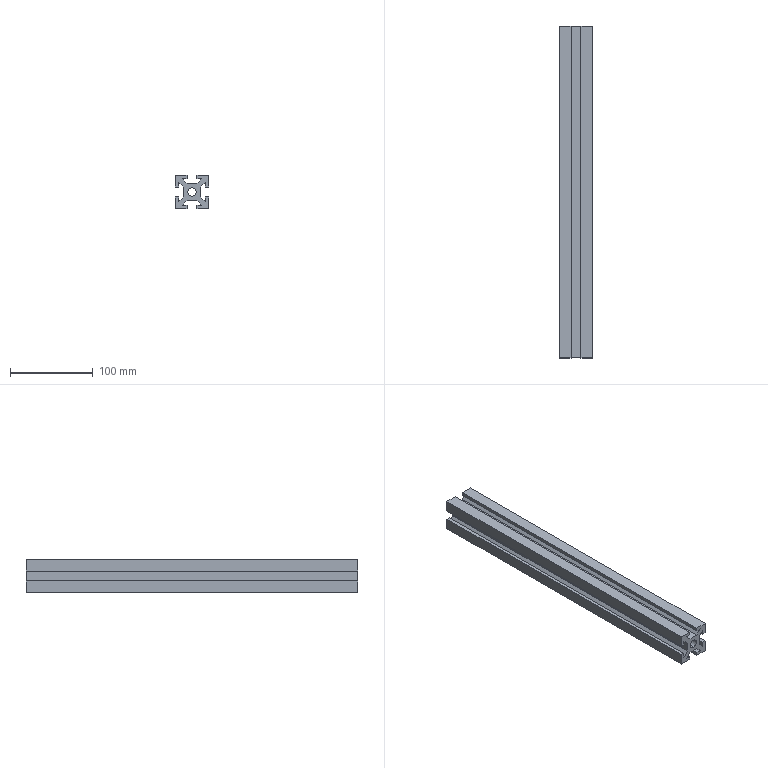Part | SolidWorks | features Extrusion 1 | 1 solid | 40 faces | box 40 x 400 x 40 mm | volume 363643 mm3 | plane 38 | cylinder 2 | commonest cylinder face diameters 10 x2
STEP:
#1=CARTESIAN_POINT('',(0.,400.,-5.));
#2=VERTEX_POINT('',#1);
#3=CARTESIAN_POINT('',(0.,400.,5.));
#4=VERTEX_POINT('',#3);
#5=CARTESIAN_POINT('',(0.,400.,0.));
#6=DIRECTION('',(0.,1.,0.));
#7=DIRECTION('',(0.,0.,1.));
#8=AXIS2_PLACEMENT_3D('',#5,#6,#7);
#9=CIRCLE('',#8,5.);
#10=EDGE_CURVE('',#2,#4,#9,.T.);
#11=ORIENTED_EDGE('',*,*,#10,.T.);
#12=CARTESIAN_POINT('',(0.,0.,5.));
#13=VERTEX_POINT('',#12);
#14=CARTESIAN_POINT('',(0.,400.,5.));
#15=DIRECTION('',(0.,-1.,0.));
#16=VECTOR('',#15,1000.);
#17=LINE('',#14,#16);
#18=EDGE_CURVE('',#4,#13,#17,.T.);
#19=ORIENTED_EDGE('',*,*,#18,.T.);
#20=CARTESIAN_POINT('',(0.,0.,-5.));
#21=VERTEX_POINT('',#20);
#22=CARTESIAN_POINT('',(0.,0.,0.));
#23=DIRECTION('',(0.,1.,0.));
#24=DIRECTION('',(0.,0.,1.));
#25=AXIS2_PLACEMENT_3D('',#22,#23,#24);
#26=CIRCLE('',#25,5.);
#27=EDGE_CURVE('',#21,#13,#26,.T.);
#28=ORIENTED_EDGE('',*,*,#27,.F.);
#29=CARTESIAN_POINT('',(0.,400.,-5.));
#30=DIRECTION('',(0.,-1.,0.));
#31=VECTOR('',#30,1000.);
#32=LINE('',#29,#31);
#33=EDGE_CURVE('',#2,#21,#32,.T.);
#34=ORIENTED_EDGE('',*,*,#33,.F.);
#35=EDGE_LOOP('',(#11,#19,#28,#34));
#36=FACE_OUTER_BOUND('',#35,.T.);
#37=CARTESIAN_POINT('',(0.,400.,0.));
#38=DIRECTION('',(0.,-1.,0.));
#39=DIRECTION('',(0.,0.,-1.));
#40=AXIS2_PLACEMENT_3D('',#37,#38,#39);
#41=CYLINDRICAL_SURFACE('',#40,5.);
#42=ADVANCED_FACE('',(#36),#41,.F.);
#43=CARTESIAN_POINT('',(6.,400.,20.));
#44=VERTEX_POINT('',#43);
#45=CARTESIAN_POINT('',(20.,400.,20.));
#46=VERTEX_POINT('',#45);
#47=CARTESIAN_POINT('',(6.,400.,20.));
#48=DIRECTION('',(1.,0.,0.));
#49=VECTOR('',#48,1000.);
#50=LINE('',#47,#49);
#51=EDGE_CURVE('',#44,#46,#50,.T.);
#52=ORIENTED_EDGE('',*,*,#51,.T.);
#53=CARTESIAN_POINT('',(20.,400.,6.));
#54=VERTEX_POINT('',#53);
#55=CARTESIAN_POINT('',(20.,400.,6.));
#56=DIRECTION('',(0.,0.,-1.));
#57=VECTOR('',#56,1000.);
#58=LINE('',#55,#57);
#59=EDGE_CURVE('',#46,#54,#58,.T.);
#60=ORIENTED_EDGE('',*,*,#59,.T.);
#61=CARTESIAN_POINT('',(16.,400.,6.));
#62=VERTEX_POINT('',#61);
#63=CARTESIAN_POINT('',(16.,400.,6.));
#64=DIRECTION('',(-1.,0.,0.));
#65=VECTOR('',#64,1000.);
#66=LINE('',#63,#65);
#67=EDGE_CURVE('',#54,#62,#66,.T.);
#68=ORIENTED_EDGE('',*,*,#67,.T.);
#69=CARTESIAN_POINT('',(16.,400.,11.757));
#70=VERTEX_POINT('',#69);
#71=CARTESIAN_POINT('',(16.,400.,11.757));
#72=DIRECTION('',(0.,0.,1.));
#73=VECTOR('',#72,1000.);
#74=LINE('',#71,#73);
#75=EDGE_CURVE('',#62,#70,#74,.T.);
#76=ORIENTED_EDGE('',*,*,#75,.T.);
#77=CARTESIAN_POINT('',(10.,400.,5.757));
#78=VERTEX_POINT('',#77);
#79=CARTESIAN_POINT('',(10.,400.,5.757));
#80=DIRECTION('',(-0.7071,0.,-0.7071));
#81=VECTOR('',#80,1000.);
#82=LINE('',#79,#81);
#83=EDGE_CURVE('',#70,#78,#82,.T.);
#84=ORIENTED_EDGE('',*,*,#83,.T.);
#85=CARTESIAN_POINT('',(10.,400.,-5.757));
#86=VERTEX_POINT('',#85);
#87=CARTESIAN_POINT('',(10.,400.,5.757));
#88=DIRECTION('',(0.,0.,-1.));
#89=VECTOR('',#88,1000.);
#90=LINE('',#87,#89);
#91=EDGE_CURVE('',#78,#86,#90,.T.);
#92=ORIENTED_EDGE('',*,*,#91,.T.);
#93=CARTESIAN_POINT('',(16.,400.,-11.757));
#94=VERTEX_POINT('',#93);
#95=CARTESIAN_POINT('',(16.,400.,-11.757));
#96=DIRECTION('',(0.7071,0.,-0.7071));
#97=VECTOR('',#96,1000.);
#98=LINE('',#95,#97);
#99=EDGE_CURVE('',#86,#94,#98,.T.);
#100=ORIENTED_EDGE('',*,*,#99,.T.);
#101=CARTESIAN_POINT('',(16.,400.,-6.));
#102=VERTEX_POINT('',#101);
#103=CARTESIAN_POINT('',(16.,400.,-6.));
#104=DIRECTION('',(0.,0.,1.));
#105=VECTOR('',#104,1000.);
#106=LINE('',#103,#105);
#107=EDGE_CURVE('',#94,#102,#106,.T.);
#108=ORIENTED_EDGE('',*,*,#107,.T.);
#109=CARTESIAN_POINT('',(20.,400.,-6.));
#110=VERTEX_POINT('',#109);
#111=CARTESIAN_POINT('',(20.,400.,-6.));
#112=DIRECTION('',(1.,0.,0.));
#113=VECTOR('',#112,1000.);
#114=LINE('',#111,#113);
#115=EDGE_CURVE('',#102,#110,#114,.T.);
#116=ORIENTED_EDGE('',*,*,#115,.T.);
#117=CARTESIAN_POINT('',(20.,400.,-20.));
#118=VERTEX_POINT('',#117);
#119=CARTESIAN_POINT('',(20.,400.,-20.));
#120=DIRECTION('',(0.,0.,-1.));
#121=VECTOR('',#120,1000.);
#122=LINE('',#119,#121);
#123=EDGE_CURVE('',#110,#118,#122,.T.);
#124=ORIENTED_EDGE('',*,*,#123,.T.);
#125=CARTESIAN_POINT('',(6.,400.,-20.));
#126=VERTEX_POINT('',#125);
#127=CARTESIAN_POINT('',(6.,400.,-20.));
#128=DIRECTION('',(-1.,0.,0.));
#129=VECTOR('',#128,1000.);
#130=LINE('',#127,#129);
#131=EDGE_CURVE('',#118,#126,#130,.T.);
#132=ORIENTED_EDGE('',*,*,#131,.T.);
#133=CARTESIAN_POINT('',(6.,400.,-16.));
#134=VERTEX_POINT('',#133);
#135=CARTESIAN_POINT('',(6.,400.,-16.));
#136=DIRECTION('',(0.,0.,1.));
#137=VECTOR('',#136,1000.);
#138=LINE('',#135,#137);
#139=EDGE_CURVE('',#126,#134,#138,.T.);
#140=ORIENTED_EDGE('',*,*,#139,.T.);
#141=CARTESIAN_POINT('',(11.757,400.,-16.));
#142=VERTEX_POINT('',#141);
#143=CARTESIAN_POINT('',(11.757,400.,-16.));
#144=DIRECTION('',(1.,0.,0.));
#145=VECTOR('',#144,1000.);
#146=LINE('',#143,#145);
#147=EDGE_CURVE('',#134,#142,#146,.T.);
#148=ORIENTED_EDGE('',*,*,#147,.T.);
#149=CARTESIAN_POINT('',(5.757,400.,-10.));
#150=VERTEX_POINT('',#149);
#151=CARTESIAN_POINT('',(5.757,400.,-10.));
#152=DIRECTION('',(-0.7071,0.,0.7071));
#153=VECTOR('',#152,1000.);
#154=LINE('',#151,#153);
#155=EDGE_CURVE('',#142,#150,#154,.T.);
#156=ORIENTED_EDGE('',*,*,#155,.T.);
#157=CARTESIAN_POINT('',(-5.757,400.,-10.));
#158=VERTEX_POINT('',#157);
#159=CARTESIAN_POINT('',(-5.757,400.,-10.));
#160=DIRECTION('',(-1.,0.,0.));
#161=VECTOR('',#160,1000.);
#162=LINE('',#159,#161);
#163=EDGE_CURVE('',#150,#158,#162,.T.);
#164=ORIENTED_EDGE('',*,*,#163,.T.);
#165=CARTESIAN_POINT('',(-11.757,400.,-16.));
#166=VERTEX_POINT('',#165);
#167=CARTESIAN_POINT('',(-11.757,400.,-16.));
#168=DIRECTION('',(-0.7071,0.,-0.7071));
#169=VECTOR('',#168,1000.);
#170=LINE('',#167,#169);
#171=EDGE_CURVE('',#158,#166,#170,.T.);
#172=ORIENTED_EDGE('',*,*,#171,.T.);
#173=CARTESIAN_POINT('',(-6.,400.,-16.));
#174=VERTEX_POINT('',#173);
#175=CARTESIAN_POINT('',(-6.,400.,-16.));
#176=DIRECTION('',(1.,0.,0.));
#177=VECTOR('',#176,1000.);
#178=LINE('',#175,#177);
#179=EDGE_CURVE('',#166,#174,#178,.T.);
#180=ORIENTED_EDGE('',*,*,#179,.T.);
#181=CARTESIAN_POINT('',(-6.,400.,-20.));
#182=VERTEX_POINT('',#181);
#183=CARTESIAN_POINT('',(-6.,400.,-20.));
#184=DIRECTION('',(0.,0.,-1.));
#185=VECTOR('',#184,1000.);
#186=LINE('',#183,#185);
#187=EDGE_CURVE('',#174,#182,#186,.T.);
#188=ORIENTED_EDGE('',*,*,#187,.T.);
#189=CARTESIAN_POINT('',(-20.,400.,-20.));
#190=VERTEX_POINT('',#189);
#191=CARTESIAN_POINT('',(-20.,400.,-20.));
#192=DIRECTION('',(-1.,0.,0.));
#193=VECTOR('',#192,1000.);
#194=LINE('',#191,#193);
#195=EDGE_CURVE('',#182,#190,#194,.T.);
#196=ORIENTED_EDGE('',*,*,#195,.T.);
#197=CARTESIAN_POINT('',(-20.,400.,-6.));
#198=VERTEX_POINT('',#197);
#199=CARTESIAN_POINT('',(-20.,400.,-20.));
#200=DIRECTION('',(0.,0.,1.));
#201=VECTOR('',#200,1000.);
#202=LINE('',#199,#201);
#203=EDGE_CURVE('',#190,#198,#202,.T.);
#204=ORIENTED_EDGE('',*,*,#203,.T.);
#205=CARTESIAN_POINT('',(-16.,400.,-6.));
#206=VERTEX_POINT('',#205);
#207=CARTESIAN_POINT('',(-16.,400.,-6.));
#208=DIRECTION('',(1.,0.,0.));
#209=VECTOR('',#208,1000.);
#210=LINE('',#207,#209);
#211=EDGE_CURVE('',#198,#206,#210,.T.);
#212=ORIENTED_EDGE('',*,*,#211,.T.);
#213=CARTESIAN_POINT('',(-16.,400.,-11.757));
#214=VERTEX_POINT('',#213);
#215=CARTESIAN_POINT('',(-16.,400.,-11.757));
#216=DIRECTION('',(0.,0.,-1.));
#217=VECTOR('',#216,1000.);
#218=LINE('',#215,#217);
#219=EDGE_CURVE('',#206,#214,#218,.T.);
#220=ORIENTED_EDGE('',*,*,#219,.T.);
#221=CARTESIAN_POINT('',(-10.,400.,-5.757));
#222=VERTEX_POINT('',#221);
#223=CARTESIAN_POINT('',(-10.,400.,-5.757));
#224=DIRECTION('',(0.7071,0.,0.7071));
#225=VECTOR('',#224,1000.);
#226=LINE('',#223,#225);
#227=EDGE_CURVE('',#214,#222,#226,.T.);
#228=ORIENTED_EDGE('',*,*,#227,.T.);
#229=CARTESIAN_POINT('',(-10.,400.,5.757));
#230=VERTEX_POINT('',#229);
#231=CARTESIAN_POINT('',(-10.,400.,5.757));
#232=DIRECTION('',(0.,0.,1.));
#233=VECTOR('',#232,1000.);
#234=LINE('',#231,#233);
#235=EDGE_CURVE('',#222,#230,#234,.T.);
#236=ORIENTED_EDGE('',*,*,#235,.T.);
#237=CARTESIAN_POINT('',(-16.,400.,11.757));
#238=VERTEX_POINT('',#237);
#239=CARTESIAN_POINT('',(-16.,400.,11.757));
#240=DIRECTION('',(-0.7071,0.,0.7071));
#241=VECTOR('',#240,1000.);
#242=LINE('',#239,#241);
#243=EDGE_CURVE('',#230,#238,#242,.T.);
#244=ORIENTED_EDGE('',*,*,#243,.T.);
#245=CARTESIAN_POINT('',(-16.,400.,6.));
#246=VERTEX_POINT('',#245);
#247=CARTESIAN_POINT('',(-16.,400.,6.));
#248=DIRECTION('',(0.,0.,-1.));
#249=VECTOR('',#248,1000.);
#250=LINE('',#247,#249);
#251=EDGE_CURVE('',#238,#246,#250,.T.);
#252=ORIENTED_EDGE('',*,*,#251,.T.);
#253=CARTESIAN_POINT('',(-20.,400.,6.));
#254=VERTEX_POINT('',#253);
#255=CARTESIAN_POINT('',(-20.,400.,6.));
#256=DIRECTION('',(-1.,0.,0.));
#257=VECTOR('',#256,1000.);
#258=LINE('',#255,#257);
#259=EDGE_CURVE('',#246,#254,#258,.T.);
#260=ORIENTED_EDGE('',*,*,#259,.T.);
#261=CARTESIAN_POINT('',(-20.,400.,20.));
#262=VERTEX_POINT('',#261);
#263=CARTESIAN_POINT('',(-20.,400.,6.));
#264=DIRECTION('',(0.,0.,1.));
#265=VECTOR('',#264,1000.);
#266=LINE('',#263,#265);
#267=EDGE_CURVE('',#254,#262,#266,.T.);
#268=ORIENTED_EDGE('',*,*,#267,.T.);
#269=CARTESIAN_POINT('',(-6.,400.,20.));
#270=VERTEX_POINT('',#269);
#271=CARTESIAN_POINT('',(-20.,400.,20.));
#272=DIRECTION('',(1.,0.,0.));
#273=VECTOR('',#272,1000.);
#274=LINE('',#271,#273);
#275=EDGE_CURVE('',#262,#270,#274,.T.);
#276=ORIENTED_EDGE('',*,*,#275,.T.);
#277=CARTESIAN_POINT('',(-6.,400.,16.));
#278=VERTEX_POINT('',#277);
#279=CARTESIAN_POINT('',(-6.,400.,16.));
#280=DIRECTION('',(0.,0.,-1.));
#281=VECTOR('',#280,1000.);
#282=LINE('',#279,#281);
#283=EDGE_CURVE('',#270,#278,#282,.T.);
#284=ORIENTED_EDGE('',*,*,#283,.T.);
#285=CARTESIAN_POINT('',(-11.757,400.,16.));
#286=VERTEX_POINT('',#285);
#287=CARTESIAN_POINT('',(-11.757,400.,16.));
#288=DIRECTION('',(-1.,0.,0.));
#289=VECTOR('',#288,1000.);
#290=LINE('',#287,#289);
#291=EDGE_CURVE('',#278,#286,#290,.T.);
#292=ORIENTED_EDGE('',*,*,#291,.T.);
#293=CARTESIAN_POINT('',(-5.757,400.,10.));
#294=VERTEX_POINT('',#293);
#295=CARTESIAN_POINT('',(-5.757,400.,10.));
#296=DIRECTION('',(0.7071,0.,-0.7071));
#297=VECTOR('',#296,1000.);
#298=LINE('',#295,#297);
#299=EDGE_CURVE('',#286,#294,#298,.T.);
#300=ORIENTED_EDGE('',*,*,#299,.T.);
#301=CARTESIAN_POINT('',(5.757,400.,10.));
#302=VERTEX_POINT('',#301);
#303=CARTESIAN_POINT('',(-5.757,400.,10.));
#304=DIRECTION('',(1.,0.,0.));
#305=VECTOR('',#304,1000.);
#306=LINE('',#303,#305);
#307=EDGE_CURVE('',#294,#302,#306,.T.);
#308=ORIENTED_EDGE('',*,*,#307,.T.);
#309=CARTESIAN_POINT('',(11.757,400.,16.));
#310=VERTEX_POINT('',#309);
#311=CARTESIAN_POINT('',(11.757,400.,16.));
#312=DIRECTION('',(0.7071,0.,0.7071));
#313=VECTOR('',#312,1000.);
#314=LINE('',#311,#313);
#315=EDGE_CURVE('',#302,#310,#314,.T.);
#316=ORIENTED_EDGE('',*,*,#315,.T.);
#317=CARTESIAN_POINT('',(6.,400.,16.));
#318=VERTEX_POINT('',#317);
#319=CARTESIAN_POINT('',(6.,400.,16.));
#320=DIRECTION('',(-1.,0.,0.));
#321=VECTOR('',#320,1000.);
#322=LINE('',#319,#321);
#323=EDGE_CURVE('',#310,#318,#322,.T.);
#324=ORIENTED_EDGE('',*,*,#323,.T.);
#325=CARTESIAN_POINT('',(6.,400.,20.));
#326=DIRECTION('',(0.,0.,1.));
#327=VECTOR('',#326,1000.);
#328=LINE('',#325,#327);
#329=EDGE_CURVE('',#318,#44,#328,.T.);
#330=ORIENTED_EDGE('',*,*,#329,.T.);
#331=EDGE_LOOP('',(#52,#60,#68,#76,#84,#92,#100,#108,#116,#124,#132,#140,#148,#156,#164,#172,#180,#188,#196,#204,#212,#220,#228,#236,#244,#252,#260,#268,#276,#284,#292,#300,#308,#316,#324,#330));
#332=FACE_OUTER_BOUND('',#331,.T.);
#333=ORIENTED_EDGE('',*,*,#10,.F.);
#334=CARTESIAN_POINT('',(0.,400.,0.));
#335=DIRECTION('',(0.,1.,0.));
#336=DIRECTION('',(0.,0.,1.));
#337=AXIS2_PLACEMENT_3D('',#334,#335,#336);
#338=CIRCLE('',#337,5.);
#339=EDGE_CURVE('',#4,#2,#338,.T.);
#340=ORIENTED_EDGE('',*,*,#339,.F.);
#341=EDGE_LOOP('',(#333,#340));
#342=FACE_BOUND('',#341,.T.);
#343=CARTESIAN_POINT('',(0.,400.,0.));
#344=DIRECTION('',(0.,-1.,0.));
#345=DIRECTION('',(0.,0.,-1.));
#346=AXIS2_PLACEMENT_3D('',#343,#344,#345);
#347=PLANE('',#346);
#348=ADVANCED_FACE('',(#332,#342),#347,.F.);
#349=CARTESIAN_POINT('',(6.,0.,20.));
#350=VERTEX_POINT('',#349);
#351=CARTESIAN_POINT('',(20.,0.,20.));
#352=VERTEX_POINT('',#351);
#353=CARTESIAN_POINT('',(6.,0.,20.));
#354=DIRECTION('',(1.,0.,0.));
#355=VECTOR('',#354,1000.);
#356=LINE('',#353,#355);
#357=EDGE_CURVE('',#350,#352,#356,.T.);
#358=ORIENTED_EDGE('',*,*,#357,.F.);
#359=CARTESIAN_POINT('',(6.,0.,16.));
#360=VERTEX_POINT('',#359);
#361=CARTESIAN_POINT('',(6.,0.,20.));
#362=DIRECTION('',(0.,0.,1.));
#363=VECTOR('',#362,1000.);
#364=LINE('',#361,#363);
#365=EDGE_CURVE('',#360,#350,#364,.T.);
#366=ORIENTED_EDGE('',*,*,#365,.F.);
#367=CARTESIAN_POINT('',(11.757,0.,16.));
#368=VERTEX_POINT('',#367);
#369=CARTESIAN_POINT('',(6.,0.,16.));
#370=DIRECTION('',(-1.,0.,0.));
#371=VECTOR('',#370,1000.);
#372=LINE('',#369,#371);
#373=EDGE_CURVE('',#368,#360,#372,.T.);
#374=ORIENTED_EDGE('',*,*,#373,.F.);
#375=CARTESIAN_POINT('',(5.757,0.,10.));
#376=VERTEX_POINT('',#375);
#377=CARTESIAN_POINT('',(11.757,0.,16.));
#378=DIRECTION('',(0.7071,0.,0.7071));
#379=VECTOR('',#378,1000.);
#380=LINE('',#377,#379);
#381=EDGE_CURVE('',#376,#368,#380,.T.);
#382=ORIENTED_EDGE('',*,*,#381,.F.);
#383=CARTESIAN_POINT('',(-5.757,0.,10.));
#384=VERTEX_POINT('',#383);
#385=CARTESIAN_POINT('',(-5.757,0.,10.));
#386=DIRECTION('',(1.,0.,0.));
#387=VECTOR('',#386,1000.);
#388=LINE('',#385,#387);
#389=EDGE_CURVE('',#384,#376,#388,.T.);
#390=ORIENTED_EDGE('',*,*,#389,.F.);
#391=CARTESIAN_POINT('',(-11.757,0.,16.));
#392=VERTEX_POINT('',#391);
#393=CARTESIAN_POINT('',(-5.757,0.,10.));
#394=DIRECTION('',(0.7071,0.,-0.7071));
#395=VECTOR('',#394,1000.);
#396=LINE('',#393,#395);
#397=EDGE_CURVE('',#392,#384,#396,.T.);
#398=ORIENTED_EDGE('',*,*,#397,.F.);
#399=CARTESIAN_POINT('',(-6.,0.,16.));
#400=VERTEX_POINT('',#399);
#401=CARTESIAN_POINT('',(-11.757,0.,16.));
#402=DIRECTION('',(-1.,0.,0.));
#403=VECTOR('',#402,1000.);
#404=LINE('',#401,#403);
#405=EDGE_CURVE('',#400,#392,#404,.T.);
#406=ORIENTED_EDGE('',*,*,#405,.F.);
#407=CARTESIAN_POINT('',(-6.,0.,20.));
#408=VERTEX_POINT('',#407);
#409=CARTESIAN_POINT('',(-6.,0.,16.));
#410=DIRECTION('',(0.,0.,-1.));
#411=VECTOR('',#410,1000.);
#412=LINE('',#409,#411);
#413=EDGE_CURVE('',#408,#400,#412,.T.);
#414=ORIENTED_EDGE('',*,*,#413,.F.);
#415=CARTESIAN_POINT('',(-20.,0.,20.));
#416=VERTEX_POINT('',#415);
#417=CARTESIAN_POINT('',(-20.,0.,20.));
#418=DIRECTION('',(1.,0.,0.));
#419=VECTOR('',#418,1000.);
#420=LINE('',#417,#419);
#421=EDGE_CURVE('',#416,#408,#420,.T.);
#422=ORIENTED_EDGE('',*,*,#421,.F.);
#423=CARTESIAN_POINT('',(-20.,0.,6.));
#424=VERTEX_POINT('',#423);
#425=CARTESIAN_POINT('',(-20.,0.,6.));
#426=DIRECTION('',(0.,0.,1.));
#427=VECTOR('',#426,1000.);
#428=LINE('',#425,#427);
#429=EDGE_CURVE('',#424,#416,#428,.T.);
#430=ORIENTED_EDGE('',*,*,#429,.F.);
#431=CARTESIAN_POINT('',(-16.,0.,6.));
#432=VERTEX_POINT('',#431);
#433=CARTESIAN_POINT('',(-20.,0.,6.));
#434=DIRECTION('',(-1.,0.,0.));
#435=VECTOR('',#434,1000.);
#436=LINE('',#433,#435);
#437=EDGE_CURVE('',#432,#424,#436,.T.);
#438=ORIENTED_EDGE('',*,*,#437,.F.);
#439=CARTESIAN_POINT('',(-16.,0.,11.757));
#440=VERTEX_POINT('',#439);
#441=CARTESIAN_POINT('',(-16.,0.,6.));
#442=DIRECTION('',(0.,0.,-1.));
#443=VECTOR('',#442,1000.);
#444=LINE('',#441,#443);
#445=EDGE_CURVE('',#440,#432,#444,.T.);
#446=ORIENTED_EDGE('',*,*,#445,.F.);
#447=CARTESIAN_POINT('',(-10.,0.,5.757));
#448=VERTEX_POINT('',#447);
#449=CARTESIAN_POINT('',(-16.,0.,11.757));
#450=DIRECTION('',(-0.7071,0.,0.7071));
#451=VECTOR('',#450,1000.);
#452=LINE('',#449,#451);
#453=EDGE_CURVE('',#448,#440,#452,.T.);
#454=ORIENTED_EDGE('',*,*,#453,.F.);
#455=CARTESIAN_POINT('',(-10.,0.,-5.757));
#456=VERTEX_POINT('',#455);
#457=CARTESIAN_POINT('',(-10.,0.,5.757));
#458=DIRECTION('',(0.,0.,1.));
#459=VECTOR('',#458,1000.);
#460=LINE('',#457,#459);
#461=EDGE_CURVE('',#456,#448,#460,.T.);
#462=ORIENTED_EDGE('',*,*,#461,.F.);
#463=CARTESIAN_POINT('',(-16.,0.,-11.757));
#464=VERTEX_POINT('',#463);
#465=CARTESIAN_POINT('',(-10.,0.,-5.757));
#466=DIRECTION('',(0.7071,0.,0.7071));
#467=VECTOR('',#466,1000.);
#468=LINE('',#465,#467);
#469=EDGE_CURVE('',#464,#456,#468,.T.);
#470=ORIENTED_EDGE('',*,*,#469,.F.);
#471=CARTESIAN_POINT('',(-16.,0.,-6.));
#472=VERTEX_POINT('',#471);
#473=CARTESIAN_POINT('',(-16.,0.,-11.757));
#474=DIRECTION('',(0.,0.,-1.));
#475=VECTOR('',#474,1000.);
#476=LINE('',#473,#475);
#477=EDGE_CURVE('',#472,#464,#476,.T.);
#478=ORIENTED_EDGE('',*,*,#477,.F.);
#479=CARTESIAN_POINT('',(-20.,0.,-6.));
#480=VERTEX_POINT('',#479);
#481=CARTESIAN_POINT('',(-16.,0.,-6.));
#482=DIRECTION('',(1.,0.,0.));
#483=VECTOR('',#482,1000.);
#484=LINE('',#481,#483);
#485=EDGE_CURVE('',#480,#472,#484,.T.);
#486=ORIENTED_EDGE('',*,*,#485,.F.);
#487=CARTESIAN_POINT('',(-20.,0.,-20.));
#488=VERTEX_POINT('',#487);
#489=CARTESIAN_POINT('',(-20.,0.,-20.));
#490=DIRECTION('',(0.,0.,1.));
#491=VECTOR('',#490,1000.);
#492=LINE('',#489,#491);
#493=EDGE_CURVE('',#488,#480,#492,.T.);
#494=ORIENTED_EDGE('',*,*,#493,.F.);
#495=CARTESIAN_POINT('',(-6.,0.,-20.));
#496=VERTEX_POINT('',#495);
#497=CARTESIAN_POINT('',(-20.,0.,-20.));
#498=DIRECTION('',(-1.,0.,0.));
#499=VECTOR('',#498,1000.);
#500=LINE('',#497,#499);
#501=EDGE_CURVE('',#496,#488,#500,.T.);
#502=ORIENTED_EDGE('',*,*,#501,.F.);
#503=CARTESIAN_POINT('',(-6.,0.,-16.));
#504=VERTEX_POINT('',#503);
#505=CARTESIAN_POINT('',(-6.,0.,-20.));
#506=DIRECTION('',(0.,0.,-1.));
#507=VECTOR('',#506,1000.);
#508=LINE('',#505,#507);
#509=EDGE_CURVE('',#504,#496,#508,.T.);
#510=ORIENTED_EDGE('',*,*,#509,.F.);
#511=CARTESIAN_POINT('',(-11.757,0.,-16.));
#512=VERTEX_POINT('',#511);
#513=CARTESIAN_POINT('',(-6.,0.,-16.));
#514=DIRECTION('',(1.,0.,0.));
#515=VECTOR('',#514,1000.);
#516=LINE('',#513,#515);
#517=EDGE_CURVE('',#512,#504,#516,.T.);
#518=ORIENTED_EDGE('',*,*,#517,.F.);
#519=CARTESIAN_POINT('',(-5.757,0.,-10.));
#520=VERTEX_POINT('',#519);
#521=CARTESIAN_POINT('',(-11.757,0.,-16.));
#522=DIRECTION('',(-0.7071,0.,-0.7071));
#523=VECTOR('',#522,1000.);
#524=LINE('',#521,#523);
#525=EDGE_CURVE('',#520,#512,#524,.T.);
#526=ORIENTED_EDGE('',*,*,#525,.F.);
#527=CARTESIAN_POINT('',(5.757,0.,-10.));
#528=VERTEX_POINT('',#527);
#529=CARTESIAN_POINT('',(-5.757,0.,-10.));
#530=DIRECTION('',(-1.,0.,0.));
#531=VECTOR('',#530,1000.);
#532=LINE('',#529,#531);
#533=EDGE_CURVE('',#528,#520,#532,.T.);
#534=ORIENTED_EDGE('',*,*,#533,.F.);
#535=CARTESIAN_POINT('',(11.757,0.,-16.));
#536=VERTEX_POINT('',#535);
#537=CARTESIAN_POINT('',(5.757,0.,-10.));
#538=DIRECTION('',(-0.7071,0.,0.7071));
#539=VECTOR('',#538,1000.);
#540=LINE('',#537,#539);
#541=EDGE_CURVE('',#536,#528,#540,.T.);
#542=ORIENTED_EDGE('',*,*,#541,.F.);
#543=CARTESIAN_POINT('',(6.,0.,-16.));
#544=VERTEX_POINT('',#543);
#545=CARTESIAN_POINT('',(11.757,0.,-16.));
#546=DIRECTION('',(1.,0.,0.));
#547=VECTOR('',#546,1000.);
#548=LINE('',#545,#547);
#549=EDGE_CURVE('',#544,#536,#548,.T.);
#550=ORIENTED_EDGE('',*,*,#549,.F.);
#551=CARTESIAN_POINT('',(6.,0.,-20.));
#552=VERTEX_POINT('',#551);
#553=CARTESIAN_POINT('',(6.,0.,-16.));
#554=DIRECTION('',(0.,0.,1.));
#555=VECTOR('',#554,1000.);
#556=LINE('',#553,#555);
#557=EDGE_CURVE('',#552,#544,#556,.T.);
#558=ORIENTED_EDGE('',*,*,#557,.F.);
#559=CARTESIAN_POINT('',(20.,0.,-20.));
#560=VERTEX_POINT('',#559);
#561=CARTESIAN_POINT('',(6.,0.,-20.));
#562=DIRECTION('',(-1.,0.,0.));
#563=VECTOR('',#562,1000.);
#564=LINE('',#561,#563);
#565=EDGE_CURVE('',#560,#552,#564,.T.);
#566=ORIENTED_EDGE('',*,*,#565,.F.);
#567=CARTESIAN_POINT('',(20.,0.,-6.));
#568=VERTEX_POINT('',#567);
#569=CARTESIAN_POINT('',(20.,0.,-20.));
#570=DIRECTION('',(0.,0.,-1.));
#571=VECTOR('',#570,1000.);
#572=LINE('',#569,#571);
#573=EDGE_CURVE('',#568,#560,#572,.T.);
#574=ORIENTED_EDGE('',*,*,#573,.F.);
#575=CARTESIAN_POINT('',(16.,0.,-6.));
#576=VERTEX_POINT('',#575);
#577=CARTESIAN_POINT('',(20.,0.,-6.));
#578=DIRECTION('',(1.,0.,0.));
#579=VECTOR('',#578,1000.);
#580=LINE('',#577,#579);
#581=EDGE_CURVE('',#576,#568,#580,.T.);
#582=ORIENTED_EDGE('',*,*,#581,.F.);
#583=CARTESIAN_POINT('',(16.,0.,-11.757));
#584=VERTEX_POINT('',#583);
#585=CARTESIAN_POINT('',(16.,0.,-6.));
#586=DIRECTION('',(0.,0.,1.));
#587=VECTOR('',#586,1000.);
#588=LINE('',#585,#587);
#589=EDGE_CURVE('',#584,#576,#588,.T.);
#590=ORIENTED_EDGE('',*,*,#589,.F.);
#591=CARTESIAN_POINT('',(10.,0.,-5.757));
#592=VERTEX_POINT('',#591);
#593=CARTESIAN_POINT('',(16.,0.,-11.757));
#594=DIRECTION('',(0.7071,0.,-0.7071));
#595=VECTOR('',#594,1000.);
#596=LINE('',#593,#595);
#597=EDGE_CURVE('',#592,#584,#596,.T.);
#598=ORIENTED_EDGE('',*,*,#597,.F.);
#599=CARTESIAN_POINT('',(10.,0.,5.757));
#600=VERTEX_POINT('',#599);
#601=CARTESIAN_POINT('',(10.,0.,5.757));
#602=DIRECTION('',(0.,0.,-1.));
#603=VECTOR('',#602,1000.);
#604=LINE('',#601,#603);
#605=EDGE_CURVE('',#600,#592,#604,.T.);
#606=ORIENTED_EDGE('',*,*,#605,.F.);
#607=CARTESIAN_POINT('',(16.,0.,11.757));
#608=VERTEX_POINT('',#607);
#609=CARTESIAN_POINT('',(10.,0.,5.757));
#610=DIRECTION('',(-0.7071,0.,-0.7071));
#611=VECTOR('',#610,1000.);
#612=LINE('',#609,#611);
#613=EDGE_CURVE('',#608,#600,#612,.T.);
#614=ORIENTED_EDGE('',*,*,#613,.F.);
#615=CARTESIAN_POINT('',(16.,0.,6.));
#616=VERTEX_POINT('',#615);
#617=CARTESIAN_POINT('',(16.,0.,11.757));
#618=DIRECTION('',(0.,0.,1.));
#619=VECTOR('',#618,1000.);
#620=LINE('',#617,#619);
#621=EDGE_CURVE('',#616,#608,#620,.T.);
#622=ORIENTED_EDGE('',*,*,#621,.F.);
#623=CARTESIAN_POINT('',(20.,0.,6.));
#624=VERTEX_POINT('',#623);
#625=CARTESIAN_POINT('',(16.,0.,6.));
#626=DIRECTION('',(-1.,0.,0.));
#627=VECTOR('',#626,1000.);
#628=LINE('',#625,#627);
#629=EDGE_CURVE('',#624,#616,#628,.T.);
#630=ORIENTED_EDGE('',*,*,#629,.F.);
#631=CARTESIAN_POINT('',(20.,0.,6.));
#632=DIRECTION('',(0.,0.,-1.));
#633=VECTOR('',#632,1000.);
#634=LINE('',#631,#633);
#635=EDGE_CURVE('',#352,#624,#634,.T.);
#636=ORIENTED_EDGE('',*,*,#635,.F.);
#637=EDGE_LOOP('',(#358,#366,#374,#382,#390,#398,#406,#414,#422,#430,#438,#446,#454,#462,#470,#478,#486,#494,#502,#510,#518,#526,#534,#542,#550,#558,#566,#574,#582,#590,#598,#606,#614,#622,#630,#636));
#638=FACE_OUTER_BOUND('',#637,.T.);
#639=ORIENTED_EDGE('',*,*,#27,.T.);
#640=CARTESIAN_POINT('',(0.,0.,0.));
#641=DIRECTION('',(0.,1.,0.));
#642=DIRECTION('',(0.,0.,1.));
#643=AXIS2_PLACEMENT_3D('',#640,#641,#642);
#644=CIRCLE('',#643,5.);
#645=EDGE_CURVE('',#13,#21,#644,.T.);
#646=ORIENTED_EDGE('',*,*,#645,.T.);
#647=EDGE_LOOP('',(#639,#646));
#648=FACE_BOUND('',#647,.T.);
#649=CARTESIAN_POINT('',(0.,0.,0.));
#650=DIRECTION('',(0.,-1.,0.));
#651=DIRECTION('',(0.,0.,-1.));
#652=AXIS2_PLACEMENT_3D('',#649,#650,#651);
#653=PLANE('',#652);
#654=ADVANCED_FACE('',(#638,#648),#653,.T.);
#655=ORIENTED_EDGE('',*,*,#357,.T.);
#656=CARTESIAN_POINT('',(20.,400.,20.));
#657=DIRECTION('',(0.,-1.,0.));
#658=VECTOR('',#657,1000.);
#659=LINE('',#656,#658);
#660=EDGE_CURVE('',#46,#352,#659,.T.);
#661=ORIENTED_EDGE('',*,*,#660,.F.);
#662=ORIENTED_EDGE('',*,*,#51,.F.);
#663=CARTESIAN_POINT('',(6.,400.,20.));
#664=DIRECTION('',(0.,-1.,0.));
#665=VECTOR('',#664,1000.);
#666=LINE('',#663,#665);
#667=EDGE_CURVE('',#44,#350,#666,.T.);
#668=ORIENTED_EDGE('',*,*,#667,.T.);
#669=EDGE_LOOP('',(#655,#661,#662,#668));
#670=FACE_OUTER_BOUND('',#669,.T.);
#671=CARTESIAN_POINT('',(6.,400.,20.));
#672=DIRECTION('',(0.,0.,-1.));
#673=DIRECTION('',(-1.,0.,0.));
#674=AXIS2_PLACEMENT_3D('',#671,#672,#673);
#675=PLANE('',#674);
#676=ADVANCED_FACE('',(#670),#675,.F.);
#677=ORIENTED_EDGE('',*,*,#635,.T.);
#678=CARTESIAN_POINT('',(20.,400.,6.));
#679=DIRECTION('',(0.,-1.,0.));
#680=VECTOR('',#679,1000.);
#681=LINE('',#678,#680);
#682=EDGE_CURVE('',#54,#624,#681,.T.);
#683=ORIENTED_EDGE('',*,*,#682,.F.);
#684=ORIENTED_EDGE('',*,*,#59,.F.);
#685=ORIENTED_EDGE('',*,*,#660,.T.);
#686=EDGE_LOOP('',(#677,#683,#684,#685));
#687=FACE_OUTER_BOUND('',#686,.T.);
#688=CARTESIAN_POINT('',(20.,400.,6.));
#689=DIRECTION('',(-1.,0.,0.));
#690=DIRECTION('',(0.,0.,1.));
#691=AXIS2_PLACEMENT_3D('',#688,#689,#690);
#692=PLANE('',#691);
#693=ADVANCED_FACE('',(#687),#692,.F.);
#694=ORIENTED_EDGE('',*,*,#629,.T.);
#695=CARTESIAN_POINT('',(16.,400.,6.));
#696=DIRECTION('',(0.,-1.,0.));
#697=VECTOR('',#696,1000.);
#698=LINE('',#695,#697);
#699=EDGE_CURVE('',#62,#616,#698,.T.);
#700=ORIENTED_EDGE('',*,*,#699,.F.);
#701=ORIENTED_EDGE('',*,*,#67,.F.);
#702=ORIENTED_EDGE('',*,*,#682,.T.);
#703=EDGE_LOOP('',(#694,#700,#701,#702));
#704=FACE_OUTER_BOUND('',#703,.T.);
#705=CARTESIAN_POINT('',(16.,400.,6.));
#706=DIRECTION('',(0.,0.,1.));
#707=DIRECTION('',(1.,0.,0.));
#708=AXIS2_PLACEMENT_3D('',#705,#706,#707);
#709=PLANE('',#708);
#710=ADVANCED_FACE('',(#704),#709,.F.);
#711=ORIENTED_EDGE('',*,*,#621,.T.);
#712=CARTESIAN_POINT('',(16.,400.,11.757));
#713=DIRECTION('',(0.,-1.,0.));
#714=VECTOR('',#713,1000.);
#715=LINE('',#712,#714);
#716=EDGE_CURVE('',#70,#608,#715,.T.);
#717=ORIENTED_EDGE('',*,*,#716,.F.);
#718=ORIENTED_EDGE('',*,*,#75,.F.);
#719=ORIENTED_EDGE('',*,*,#699,.T.);
#720=EDGE_LOOP('',(#711,#717,#718,#719));
#721=FACE_OUTER_BOUND('',#720,.T.);
#722=CARTESIAN_POINT('',(16.,400.,11.757));
#723=DIRECTION('',(1.,0.,0.));
#724=DIRECTION('',(0.,0.,-1.));
#725=AXIS2_PLACEMENT_3D('',#722,#723,#724);
#726=PLANE('',#725);
#727=ADVANCED_FACE('',(#721),#726,.F.);
#728=ORIENTED_EDGE('',*,*,#613,.T.);
#729=CARTESIAN_POINT('',(10.,400.,5.757));
#730=DIRECTION('',(0.,-1.,0.));
#731=VECTOR('',#730,1000.);
#732=LINE('',#729,#731);
#733=EDGE_CURVE('',#78,#600,#732,.T.);
#734=ORIENTED_EDGE('',*,*,#733,.F.);
#735=ORIENTED_EDGE('',*,*,#83,.F.);
#736=ORIENTED_EDGE('',*,*,#716,.T.);
#737=EDGE_LOOP('',(#728,#734,#735,#736));
#738=FACE_OUTER_BOUND('',#737,.T.);
#739=CARTESIAN_POINT('',(10.,400.,5.757));
#740=DIRECTION('',(-0.7071,0.,0.7071));
#741=DIRECTION('',(0.7071,0.,0.7071));
#742=AXIS2_PLACEMENT_3D('',#739,#740,#741);
#743=PLANE('',#742);
#744=ADVANCED_FACE('',(#738),#743,.F.);
#745=ORIENTED_EDGE('',*,*,#605,.T.);
#746=CARTESIAN_POINT('',(10.,400.,-5.757));
#747=DIRECTION('',(0.,-1.,0.));
#748=VECTOR('',#747,1000.);
#749=LINE('',#746,#748);
#750=EDGE_CURVE('',#86,#592,#749,.T.);
#751=ORIENTED_EDGE('',*,*,#750,.F.);
#752=ORIENTED_EDGE('',*,*,#91,.F.);
#753=ORIENTED_EDGE('',*,*,#733,.T.);
#754=EDGE_LOOP('',(#745,#751,#752,#753));
#755=FACE_OUTER_BOUND('',#754,.T.);
#756=CARTESIAN_POINT('',(10.,400.,5.757));
#757=DIRECTION('',(-1.,0.,0.));
#758=DIRECTION('',(0.,0.,1.));
#759=AXIS2_PLACEMENT_3D('',#756,#757,#758);
#760=PLANE('',#759);
#761=ADVANCED_FACE('',(#755),#760,.F.);
#762=ORIENTED_EDGE('',*,*,#597,.T.);
#763=CARTESIAN_POINT('',(16.,400.,-11.757));
#764=DIRECTION('',(0.,-1.,0.));
#765=VECTOR('',#764,1000.);
#766=LINE('',#763,#765);
#767=EDGE_CURVE('',#94,#584,#766,.T.);
#768=ORIENTED_EDGE('',*,*,#767,.F.);
#769=ORIENTED_EDGE('',*,*,#99,.F.);
#770=ORIENTED_EDGE('',*,*,#750,.T.);
#771=EDGE_LOOP('',(#762,#768,#769,#770));
#772=FACE_OUTER_BOUND('',#771,.T.);
#773=CARTESIAN_POINT('',(16.,400.,-11.757));
#774=DIRECTION('',(-0.7071,0.,-0.7071));
#775=DIRECTION('',(-0.7071,0.,0.7071));
#776=AXIS2_PLACEMENT_3D('',#773,#774,#775);
#777=PLANE('',#776);
#778=ADVANCED_FACE('',(#772),#777,.F.);
#779=ORIENTED_EDGE('',*,*,#589,.T.);
#780=CARTESIAN_POINT('',(16.,400.,-6.));
#781=DIRECTION('',(0.,-1.,0.));
#782=VECTOR('',#781,1000.);
#783=LINE('',#780,#782);
#784=EDGE_CURVE('',#102,#576,#783,.T.);
#785=ORIENTED_EDGE('',*,*,#784,.F.);
#786=ORIENTED_EDGE('',*,*,#107,.F.);
#787=ORIENTED_EDGE('',*,*,#767,.T.);
#788=EDGE_LOOP('',(#779,#785,#786,#787));
#789=FACE_OUTER_BOUND('',#788,.T.);
#790=CARTESIAN_POINT('',(16.,400.,-6.));
#791=DIRECTION('',(1.,0.,0.));
#792=DIRECTION('',(0.,0.,-1.));
#793=AXIS2_PLACEMENT_3D('',#790,#791,#792);
#794=PLANE('',#793);
#795=ADVANCED_FACE('',(#789),#794,.F.);
#796=ORIENTED_EDGE('',*,*,#581,.T.);
#797=CARTESIAN_POINT('',(20.,400.,-6.));
#798=DIRECTION('',(0.,-1.,0.));
#799=VECTOR('',#798,1000.);
#800=LINE('',#797,#799);
#801=EDGE_CURVE('',#110,#568,#800,.T.);
#802=ORIENTED_EDGE('',*,*,#801,.F.);
#803=ORIENTED_EDGE('',*,*,#115,.F.);
#804=ORIENTED_EDGE('',*,*,#784,.T.);
#805=EDGE_LOOP('',(#796,#802,#803,#804));
#806=FACE_OUTER_BOUND('',#805,.T.);
#807=CARTESIAN_POINT('',(20.,400.,-6.));
#808=DIRECTION('',(0.,0.,-1.));
#809=DIRECTION('',(-1.,0.,0.));
#810=AXIS2_PLACEMENT_3D('',#807,#808,#809);
#811=PLANE('',#810);
#812=ADVANCED_FACE('',(#806),#811,.F.);
#813=ORIENTED_EDGE('',*,*,#573,.T.);
#814=CARTESIAN_POINT('',(20.,400.,-20.));
#815=DIRECTION('',(0.,-1.,0.));
#816=VECTOR('',#815,1000.);
#817=LINE('',#814,#816);
#818=EDGE_CURVE('',#118,#560,#817,.T.);
#819=ORIENTED_EDGE('',*,*,#818,.F.);
#820=ORIENTED_EDGE('',*,*,#123,.F.);
#821=ORIENTED_EDGE('',*,*,#801,.T.);
#822=EDGE_LOOP('',(#813,#819,#820,#821));
#823=FACE_OUTER_BOUND('',#822,.T.);
#824=CARTESIAN_POINT('',(20.,400.,-20.));
#825=DIRECTION('',(-1.,0.,0.));
#826=DIRECTION('',(0.,0.,1.));
#827=AXIS2_PLACEMENT_3D('',#824,#825,#826);
#828=PLANE('',#827);
#829=ADVANCED_FACE('',(#823),#828,.F.);
#830=ORIENTED_EDGE('',*,*,#565,.T.);
#831=CARTESIAN_POINT('',(6.,400.,-20.));
#832=DIRECTION('',(0.,-1.,0.));
#833=VECTOR('',#832,1000.);
#834=LINE('',#831,#833);
#835=EDGE_CURVE('',#126,#552,#834,.T.);
#836=ORIENTED_EDGE('',*,*,#835,.F.);
#837=ORIENTED_EDGE('',*,*,#131,.F.);
#838=ORIENTED_EDGE('',*,*,#818,.T.);
#839=EDGE_LOOP('',(#830,#836,#837,#838));
#840=FACE_OUTER_BOUND('',#839,.T.);
#841=CARTESIAN_POINT('',(6.,400.,-20.));
#842=DIRECTION('',(0.,0.,1.));
#843=DIRECTION('',(1.,0.,0.));
#844=AXIS2_PLACEMENT_3D('',#841,#842,#843);
#845=PLANE('',#844);
#846=ADVANCED_FACE('',(#840),#845,.F.);
#847=ORIENTED_EDGE('',*,*,#557,.T.);
#848=CARTESIAN_POINT('',(6.,400.,-16.));
#849=DIRECTION('',(0.,-1.,0.));
#850=VECTOR('',#849,1000.);
#851=LINE('',#848,#850);
#852=EDGE_CURVE('',#134,#544,#851,.T.);
#853=ORIENTED_EDGE('',*,*,#852,.F.);
#854=ORIENTED_EDGE('',*,*,#139,.F.);
#855=ORIENTED_EDGE('',*,*,#835,.T.);
#856=EDGE_LOOP('',(#847,#853,#854,#855));
#857=FACE_OUTER_BOUND('',#856,.T.);
#858=CARTESIAN_POINT('',(6.,400.,-16.));
#859=DIRECTION('',(1.,0.,0.));
#860=DIRECTION('',(0.,0.,-1.));
#861=AXIS2_PLACEMENT_3D('',#858,#859,#860);
#862=PLANE('',#861);
#863=ADVANCED_FACE('',(#857),#862,.F.);
#864=ORIENTED_EDGE('',*,*,#549,.T.);
#865=CARTESIAN_POINT('',(11.757,400.,-16.));
#866=DIRECTION('',(0.,-1.,0.));
#867=VECTOR('',#866,1000.);
#868=LINE('',#865,#867);
#869=EDGE_CURVE('',#142,#536,#868,.T.);
#870=ORIENTED_EDGE('',*,*,#869,.F.);
#871=ORIENTED_EDGE('',*,*,#147,.F.);
#872=ORIENTED_EDGE('',*,*,#852,.T.);
#873=EDGE_LOOP('',(#864,#870,#871,#872));
#874=FACE_OUTER_BOUND('',#873,.T.);
#875=CARTESIAN_POINT('',(11.757,400.,-16.));
#876=DIRECTION('',(0.,0.,-1.));
#877=DIRECTION('',(-1.,0.,0.));
#878=AXIS2_PLACEMENT_3D('',#875,#876,#877);
#879=PLANE('',#878);
#880=ADVANCED_FACE('',(#874),#879,.F.);
#881=ORIENTED_EDGE('',*,*,#541,.T.);
#882=CARTESIAN_POINT('',(5.757,400.,-10.));
#883=DIRECTION('',(0.,-1.,0.));
#884=VECTOR('',#883,1000.);
#885=LINE('',#882,#884);
#886=EDGE_CURVE('',#150,#528,#885,.T.);
#887=ORIENTED_EDGE('',*,*,#886,.F.);
#888=ORIENTED_EDGE('',*,*,#155,.F.);
#889=ORIENTED_EDGE('',*,*,#869,.T.);
#890=EDGE_LOOP('',(#881,#887,#888,#889));
#891=FACE_OUTER_BOUND('',#890,.T.);
#892=CARTESIAN_POINT('',(5.757,400.,-10.));
#893=DIRECTION('',(0.7071,0.,0.7071));
#894=DIRECTION('',(0.7071,0.,-0.7071));
#895=AXIS2_PLACEMENT_3D('',#892,#893,#894);
#896=PLANE('',#895);
#897=ADVANCED_FACE('',(#891),#896,.F.);
#898=ORIENTED_EDGE('',*,*,#533,.T.);
#899=CARTESIAN_POINT('',(-5.757,400.,-10.));
#900=DIRECTION('',(0.,-1.,0.));
#901=VECTOR('',#900,1000.);
#902=LINE('',#899,#901);
#903=EDGE_CURVE('',#158,#520,#902,.T.);
#904=ORIENTED_EDGE('',*,*,#903,.F.);
#905=ORIENTED_EDGE('',*,*,#163,.F.);
#906=ORIENTED_EDGE('',*,*,#886,.T.);
#907=EDGE_LOOP('',(#898,#904,#905,#906));
#908=FACE_OUTER_BOUND('',#907,.T.);
#909=CARTESIAN_POINT('',(-5.757,400.,-10.));
#910=DIRECTION('',(0.,0.,1.));
#911=DIRECTION('',(1.,0.,0.));
#912=AXIS2_PLACEMENT_3D('',#909,#910,#911);
#913=PLANE('',#912);
#914=ADVANCED_FACE('',(#908),#913,.F.);
#915=ORIENTED_EDGE('',*,*,#525,.T.);
#916=CARTESIAN_POINT('',(-11.757,400.,-16.));
#917=DIRECTION('',(0.,-1.,0.));
#918=VECTOR('',#917,1000.);
#919=LINE('',#916,#918);
#920=EDGE_CURVE('',#166,#512,#919,.T.);
#921=ORIENTED_EDGE('',*,*,#920,.F.);
#922=ORIENTED_EDGE('',*,*,#171,.F.);
#923=ORIENTED_EDGE('',*,*,#903,.T.);
#924=EDGE_LOOP('',(#915,#921,#922,#923));
#925=FACE_OUTER_BOUND('',#924,.T.);
#926=CARTESIAN_POINT('',(-11.757,400.,-16.));
#927=DIRECTION('',(-0.7071,0.,0.7071));
#928=DIRECTION('',(0.7071,0.,0.7071));
#929=AXIS2_PLACEMENT_3D('',#926,#927,#928);
#930=PLANE('',#929);
#931=ADVANCED_FACE('',(#925),#930,.F.);
#932=ORIENTED_EDGE('',*,*,#517,.T.);
#933=CARTESIAN_POINT('',(-6.,400.,-16.));
#934=DIRECTION('',(0.,-1.,0.));
#935=VECTOR('',#934,1000.);
#936=LINE('',#933,#935);
#937=EDGE_CURVE('',#174,#504,#936,.T.);
#938=ORIENTED_EDGE('',*,*,#937,.F.);
#939=ORIENTED_EDGE('',*,*,#179,.F.);
#940=ORIENTED_EDGE('',*,*,#920,.T.);
#941=EDGE_LOOP('',(#932,#938,#939,#940));
#942=FACE_OUTER_BOUND('',#941,.T.);
#943=CARTESIAN_POINT('',(-6.,400.,-16.));
#944=DIRECTION('',(0.,0.,-1.));
#945=DIRECTION('',(-1.,0.,0.));
#946=AXIS2_PLACEMENT_3D('',#943,#944,#945);
#947=PLANE('',#946);
#948=ADVANCED_FACE('',(#942),#947,.F.);
#949=ORIENTED_EDGE('',*,*,#509,.T.);
#950=CARTESIAN_POINT('',(-6.,400.,-20.));
#951=DIRECTION('',(0.,-1.,0.));
#952=VECTOR('',#951,1000.);
#953=LINE('',#950,#952);
#954=EDGE_CURVE('',#182,#496,#953,.T.);
#955=ORIENTED_EDGE('',*,*,#954,.F.);
#956=ORIENTED_EDGE('',*,*,#187,.F.);
#957=ORIENTED_EDGE('',*,*,#937,.T.);
#958=EDGE_LOOP('',(#949,#955,#956,#957));
#959=FACE_OUTER_BOUND('',#958,.T.);
#960=CARTESIAN_POINT('',(-6.,400.,-20.));
#961=DIRECTION('',(-1.,0.,0.));
#962=DIRECTION('',(0.,0.,1.));
#963=AXIS2_PLACEMENT_3D('',#960,#961,#962);
#964=PLANE('',#963);
#965=ADVANCED_FACE('',(#959),#964,.F.);
#966=ORIENTED_EDGE('',*,*,#501,.T.);
#967=CARTESIAN_POINT('',(-20.,400.,-20.));
#968=DIRECTION('',(0.,-1.,0.));
#969=VECTOR('',#968,1000.);
#970=LINE('',#967,#969);
#971=EDGE_CURVE('',#190,#488,#970,.T.);
#972=ORIENTED_EDGE('',*,*,#971,.F.);
#973=ORIENTED_EDGE('',*,*,#195,.F.);
#974=ORIENTED_EDGE('',*,*,#954,.T.);
#975=EDGE_LOOP('',(#966,#972,#973,#974));
#976=FACE_OUTER_BOUND('',#975,.T.);
#977=CARTESIAN_POINT('',(-20.,400.,-20.));
#978=DIRECTION('',(0.,0.,1.));
#979=DIRECTION('',(1.,0.,0.));
#980=AXIS2_PLACEMENT_3D('',#977,#978,#979);
#981=PLANE('',#980);
#982=ADVANCED_FACE('',(#976),#981,.F.);
#983=ORIENTED_EDGE('',*,*,#493,.T.);
#984=CARTESIAN_POINT('',(-20.,400.,-6.));
#985=DIRECTION('',(0.,-1.,0.));
#986=VECTOR('',#985,1000.);
#987=LINE('',#984,#986);
#988=EDGE_CURVE('',#198,#480,#987,.T.);
#989=ORIENTED_EDGE('',*,*,#988,.F.);
#990=ORIENTED_EDGE('',*,*,#203,.F.);
#991=ORIENTED_EDGE('',*,*,#971,.T.);
#992=EDGE_LOOP('',(#983,#989,#990,#991));
#993=FACE_OUTER_BOUND('',#992,.T.);
#994=CARTESIAN_POINT('',(-20.,400.,-20.));
#995=DIRECTION('',(1.,0.,0.));
#996=DIRECTION('',(0.,0.,-1.));
#997=AXIS2_PLACEMENT_3D('',#994,#995,#996);
#998=PLANE('',#997);
#999=ADVANCED_FACE('',(#993),#998,.F.);
#1000=ORIENTED_EDGE('',*,*,#485,.T.);
#1001=CARTESIAN_POINT('',(-16.,400.,-6.));
#1002=DIRECTION('',(0.,-1.,0.));
#1003=VECTOR('',#1002,1000.);
#1004=LINE('',#1001,#1003);
#1005=EDGE_CURVE('',#206,#472,#1004,.T.);
#1006=ORIENTED_EDGE('',*,*,#1005,.F.);
#1007=ORIENTED_EDGE('',*,*,#211,.F.);
#1008=ORIENTED_EDGE('',*,*,#988,.T.);
#1009=EDGE_LOOP('',(#1000,#1006,#1007,#1008));
#1010=FACE_OUTER_BOUND('',#1009,.T.);
#1011=CARTESIAN_POINT('',(-16.,400.,-6.));
#1012=DIRECTION('',(0.,0.,-1.));
#1013=DIRECTION('',(-1.,0.,0.));
#1014=AXIS2_PLACEMENT_3D('',#1011,#1012,#1013);
#1015=PLANE('',#1014);
#1016=ADVANCED_FACE('',(#1010),#1015,.F.);
#1017=ORIENTED_EDGE('',*,*,#477,.T.);
#1018=CARTESIAN_POINT('',(-16.,400.,-11.757));
#1019=DIRECTION('',(0.,-1.,0.));
#1020=VECTOR('',#1019,1000.);
#1021=LINE('',#1018,#1020);
#1022=EDGE_CURVE('',#214,#464,#1021,.T.);
#1023=ORIENTED_EDGE('',*,*,#1022,.F.);
#1024=ORIENTED_EDGE('',*,*,#219,.F.);
#1025=ORIENTED_EDGE('',*,*,#1005,.T.);
#1026=EDGE_LOOP('',(#1017,#1023,#1024,#1025));
#1027=FACE_OUTER_BOUND('',#1026,.T.);
#1028=CARTESIAN_POINT('',(-16.,400.,-11.757));
#1029=DIRECTION('',(-1.,0.,0.));
#1030=DIRECTION('',(0.,0.,1.));
#1031=AXIS2_PLACEMENT_3D('',#1028,#1029,#1030);
#1032=PLANE('',#1031);
#1033=ADVANCED_FACE('',(#1027),#1032,.F.);
#1034=ORIENTED_EDGE('',*,*,#469,.T.);
#1035=CARTESIAN_POINT('',(-10.,400.,-5.757));
#1036=DIRECTION('',(0.,-1.,0.));
#1037=VECTOR('',#1036,1000.);
#1038=LINE('',#1035,#1037);
#1039=EDGE_CURVE('',#222,#456,#1038,.T.);
#1040=ORIENTED_EDGE('',*,*,#1039,.F.);
#1041=ORIENTED_EDGE('',*,*,#227,.F.);
#1042=ORIENTED_EDGE('',*,*,#1022,.T.);
#1043=EDGE_LOOP('',(#1034,#1040,#1041,#1042));
#1044=FACE_OUTER_BOUND('',#1043,.T.);
#1045=CARTESIAN_POINT('',(-10.,400.,-5.757));
#1046=DIRECTION('',(0.7071,0.,-0.7071));
#1047=DIRECTION('',(-0.7071,0.,-0.7071));
#1048=AXIS2_PLACEMENT_3D('',#1045,#1046,#1047);
#1049=PLANE('',#1048);
#1050=ADVANCED_FACE('',(#1044),#1049,.F.);
#1051=ORIENTED_EDGE('',*,*,#461,.T.);
#1052=CARTESIAN_POINT('',(-10.,400.,5.757));
#1053=DIRECTION('',(0.,-1.,0.));
#1054=VECTOR('',#1053,1000.);
#1055=LINE('',#1052,#1054);
#1056=EDGE_CURVE('',#230,#448,#1055,.T.);
#1057=ORIENTED_EDGE('',*,*,#1056,.F.);
#1058=ORIENTED_EDGE('',*,*,#235,.F.);
#1059=ORIENTED_EDGE('',*,*,#1039,.T.);
#1060=EDGE_LOOP('',(#1051,#1057,#1058,#1059));
#1061=FACE_OUTER_BOUND('',#1060,.T.);
#1062=CARTESIAN_POINT('',(-10.,400.,5.757));
#1063=DIRECTION('',(1.,0.,0.));
#1064=DIRECTION('',(0.,0.,-1.));
#1065=AXIS2_PLACEMENT_3D('',#1062,#1063,#1064);
#1066=PLANE('',#1065);
#1067=ADVANCED_FACE('',(#1061),#1066,.F.);
#1068=ORIENTED_EDGE('',*,*,#453,.T.);
#1069=CARTESIAN_POINT('',(-16.,400.,11.757));
#1070=DIRECTION('',(0.,-1.,0.));
#1071=VECTOR('',#1070,1000.);
#1072=LINE('',#1069,#1071);
#1073=EDGE_CURVE('',#238,#440,#1072,.T.);
#1074=ORIENTED_EDGE('',*,*,#1073,.F.);
#1075=ORIENTED_EDGE('',*,*,#243,.F.);
#1076=ORIENTED_EDGE('',*,*,#1056,.T.);
#1077=EDGE_LOOP('',(#1068,#1074,#1075,#1076));
#1078=FACE_OUTER_BOUND('',#1077,.T.);
#1079=CARTESIAN_POINT('',(-16.,400.,11.757));
#1080=DIRECTION('',(0.7071,0.,0.7071));
#1081=DIRECTION('',(0.7071,0.,-0.7071));
#1082=AXIS2_PLACEMENT_3D('',#1079,#1080,#1081);
#1083=PLANE('',#1082);
#1084=ADVANCED_FACE('',(#1078),#1083,.F.);
#1085=ORIENTED_EDGE('',*,*,#445,.T.);
#1086=CARTESIAN_POINT('',(-16.,400.,6.));
#1087=DIRECTION('',(0.,-1.,0.));
#1088=VECTOR('',#1087,1000.);
#1089=LINE('',#1086,#1088);
#1090=EDGE_CURVE('',#246,#432,#1089,.T.);
#1091=ORIENTED_EDGE('',*,*,#1090,.F.);
#1092=ORIENTED_EDGE('',*,*,#251,.F.);
#1093=ORIENTED_EDGE('',*,*,#1073,.T.);
#1094=EDGE_LOOP('',(#1085,#1091,#1092,#1093));
#1095=FACE_OUTER_BOUND('',#1094,.T.);
#1096=CARTESIAN_POINT('',(-16.,400.,6.));
#1097=DIRECTION('',(-1.,0.,0.));
#1098=DIRECTION('',(0.,0.,1.));
#1099=AXIS2_PLACEMENT_3D('',#1096,#1097,#1098);
#1100=PLANE('',#1099);
#1101=ADVANCED_FACE('',(#1095),#1100,.F.);
#1102=ORIENTED_EDGE('',*,*,#437,.T.);
#1103=CARTESIAN_POINT('',(-20.,400.,6.));
#1104=DIRECTION('',(0.,-1.,0.));
#1105=VECTOR('',#1104,1000.);
#1106=LINE('',#1103,#1105);
#1107=EDGE_CURVE('',#254,#424,#1106,.T.);
#1108=ORIENTED_EDGE('',*,*,#1107,.F.);
#1109=ORIENTED_EDGE('',*,*,#259,.F.);
#1110=ORIENTED_EDGE('',*,*,#1090,.T.);
#1111=EDGE_LOOP('',(#1102,#1108,#1109,#1110));
#1112=FACE_OUTER_BOUND('',#1111,.T.);
#1113=CARTESIAN_POINT('',(-20.,400.,6.));
#1114=DIRECTION('',(0.,0.,1.));
#1115=DIRECTION('',(1.,0.,0.));
#1116=AXIS2_PLACEMENT_3D('',#1113,#1114,#1115);
#1117=PLANE('',#1116);
#1118=ADVANCED_FACE('',(#1112),#1117,.F.);
#1119=ORIENTED_EDGE('',*,*,#429,.T.);
#1120=CARTESIAN_POINT('',(-20.,400.,20.));
#1121=DIRECTION('',(0.,-1.,0.));
#1122=VECTOR('',#1121,1000.);
#1123=LINE('',#1120,#1122);
#1124=EDGE_CURVE('',#262,#416,#1123,.T.);
#1125=ORIENTED_EDGE('',*,*,#1124,.F.);
#1126=ORIENTED_EDGE('',*,*,#267,.F.);
#1127=ORIENTED_EDGE('',*,*,#1107,.T.);
#1128=EDGE_LOOP('',(#1119,#1125,#1126,#1127));
#1129=FACE_OUTER_BOUND('',#1128,.T.);
#1130=CARTESIAN_POINT('',(-20.,400.,6.));
#1131=DIRECTION('',(1.,0.,0.));
#1132=DIRECTION('',(0.,0.,-1.));
#1133=AXIS2_PLACEMENT_3D('',#1130,#1131,#1132);
#1134=PLANE('',#1133);
#1135=ADVANCED_FACE('',(#1129),#1134,.F.);
#1136=ORIENTED_EDGE('',*,*,#421,.T.);
#1137=CARTESIAN_POINT('',(-6.,400.,20.));
#1138=DIRECTION('',(0.,-1.,0.));
#1139=VECTOR('',#1138,1000.);
#1140=LINE('',#1137,#1139);
#1141=EDGE_CURVE('',#270,#408,#1140,.T.);
#1142=ORIENTED_EDGE('',*,*,#1141,.F.);
#1143=ORIENTED_EDGE('',*,*,#275,.F.);
#1144=ORIENTED_EDGE('',*,*,#1124,.T.);
#1145=EDGE_LOOP('',(#1136,#1142,#1143,#1144));
#1146=FACE_OUTER_BOUND('',#1145,.T.);
#1147=CARTESIAN_POINT('',(-20.,400.,20.));
#1148=DIRECTION('',(0.,0.,-1.));
#1149=DIRECTION('',(-1.,0.,0.));
#1150=AXIS2_PLACEMENT_3D('',#1147,#1148,#1149);
#1151=PLANE('',#1150);
#1152=ADVANCED_FACE('',(#1146),#1151,.F.);
#1153=ORIENTED_EDGE('',*,*,#413,.T.);
#1154=CARTESIAN_POINT('',(-6.,400.,16.));
#1155=DIRECTION('',(0.,-1.,0.));
#1156=VECTOR('',#1155,1000.);
#1157=LINE('',#1154,#1156);
#1158=EDGE_CURVE('',#278,#400,#1157,.T.);
#1159=ORIENTED_EDGE('',*,*,#1158,.F.);
#1160=ORIENTED_EDGE('',*,*,#283,.F.);
#1161=ORIENTED_EDGE('',*,*,#1141,.T.);
#1162=EDGE_LOOP('',(#1153,#1159,#1160,#1161));
#1163=FACE_OUTER_BOUND('',#1162,.T.);
#1164=CARTESIAN_POINT('',(-6.,400.,16.));
#1165=DIRECTION('',(-1.,0.,0.));
#1166=DIRECTION('',(0.,0.,1.));
#1167=AXIS2_PLACEMENT_3D('',#1164,#1165,#1166);
#1168=PLANE('',#1167);
#1169=ADVANCED_FACE('',(#1163),#1168,.F.);
#1170=ORIENTED_EDGE('',*,*,#405,.T.);
#1171=CARTESIAN_POINT('',(-11.757,400.,16.));
#1172=DIRECTION('',(0.,-1.,0.));
#1173=VECTOR('',#1172,1000.);
#1174=LINE('',#1171,#1173);
#1175=EDGE_CURVE('',#286,#392,#1174,.T.);
#1176=ORIENTED_EDGE('',*,*,#1175,.F.);
#1177=ORIENTED_EDGE('',*,*,#291,.F.);
#1178=ORIENTED_EDGE('',*,*,#1158,.T.);
#1179=EDGE_LOOP('',(#1170,#1176,#1177,#1178));
#1180=FACE_OUTER_BOUND('',#1179,.T.);
#1181=CARTESIAN_POINT('',(-11.757,400.,16.));
#1182=DIRECTION('',(0.,0.,1.));
#1183=DIRECTION('',(1.,0.,0.));
#1184=AXIS2_PLACEMENT_3D('',#1181,#1182,#1183);
#1185=PLANE('',#1184);
#1186=ADVANCED_FACE('',(#1180),#1185,.F.);
#1187=ORIENTED_EDGE('',*,*,#397,.T.);
#1188=CARTESIAN_POINT('',(-5.757,400.,10.));
#1189=DIRECTION('',(0.,-1.,0.));
#1190=VECTOR('',#1189,1000.);
#1191=LINE('',#1188,#1190);
#1192=EDGE_CURVE('',#294,#384,#1191,.T.);
#1193=ORIENTED_EDGE('',*,*,#1192,.F.);
#1194=ORIENTED_EDGE('',*,*,#299,.F.);
#1195=ORIENTED_EDGE('',*,*,#1175,.T.);
#1196=EDGE_LOOP('',(#1187,#1193,#1194,#1195));
#1197=FACE_OUTER_BOUND('',#1196,.T.);
#1198=CARTESIAN_POINT('',(-5.757,400.,10.));
#1199=DIRECTION('',(-0.7071,0.,-0.7071));
#1200=DIRECTION('',(-0.7071,0.,0.7071));
#1201=AXIS2_PLACEMENT_3D('',#1198,#1199,#1200);
#1202=PLANE('',#1201);
#1203=ADVANCED_FACE('',(#1197),#1202,.F.);
#1204=ORIENTED_EDGE('',*,*,#389,.T.);
#1205=CARTESIAN_POINT('',(5.757,400.,10.));
#1206=DIRECTION('',(0.,-1.,0.));
#1207=VECTOR('',#1206,1000.);
#1208=LINE('',#1205,#1207);
#1209=EDGE_CURVE('',#302,#376,#1208,.T.);
#1210=ORIENTED_EDGE('',*,*,#1209,.F.);
#1211=ORIENTED_EDGE('',*,*,#307,.F.);
#1212=ORIENTED_EDGE('',*,*,#1192,.T.);
#1213=EDGE_LOOP('',(#1204,#1210,#1211,#1212));
#1214=FACE_OUTER_BOUND('',#1213,.T.);
#1215=CARTESIAN_POINT('',(-5.757,400.,10.));
#1216=DIRECTION('',(0.,0.,-1.));
#1217=DIRECTION('',(-1.,0.,0.));
#1218=AXIS2_PLACEMENT_3D('',#1215,#1216,#1217);
#1219=PLANE('',#1218);
#1220=ADVANCED_FACE('',(#1214),#1219,.F.);
#1221=ORIENTED_EDGE('',*,*,#381,.T.);
#1222=CARTESIAN_POINT('',(11.757,400.,16.));
#1223=DIRECTION('',(0.,-1.,0.));
#1224=VECTOR('',#1223,1000.);
#1225=LINE('',#1222,#1224);
#1226=EDGE_CURVE('',#310,#368,#1225,.T.);
#1227=ORIENTED_EDGE('',*,*,#1226,.F.);
#1228=ORIENTED_EDGE('',*,*,#315,.F.);
#1229=ORIENTED_EDGE('',*,*,#1209,.T.);
#1230=EDGE_LOOP('',(#1221,#1227,#1228,#1229));
#1231=FACE_OUTER_BOUND('',#1230,.T.);
#1232=CARTESIAN_POINT('',(11.757,400.,16.));
#1233=DIRECTION('',(0.7071,0.,-0.7071));
#1234=DIRECTION('',(-0.7071,0.,-0.7071));
#1235=AXIS2_PLACEMENT_3D('',#1232,#1233,#1234);
#1236=PLANE('',#1235);
#1237=ADVANCED_FACE('',(#1231),#1236,.F.);
#1238=ORIENTED_EDGE('',*,*,#373,.T.);
#1239=CARTESIAN_POINT('',(6.,400.,16.));
#1240=DIRECTION('',(0.,-1.,0.));
#1241=VECTOR('',#1240,1000.);
#1242=LINE('',#1239,#1241);
#1243=EDGE_CURVE('',#318,#360,#1242,.T.);
#1244=ORIENTED_EDGE('',*,*,#1243,.F.);
#1245=ORIENTED_EDGE('',*,*,#323,.F.);
#1246=ORIENTED_EDGE('',*,*,#1226,.T.);
#1247=EDGE_LOOP('',(#1238,#1244,#1245,#1246));
#1248=FACE_OUTER_BOUND('',#1247,.T.);
#1249=CARTESIAN_POINT('',(6.,400.,16.));
#1250=DIRECTION('',(0.,0.,1.));
#1251=DIRECTION('',(1.,0.,0.));
#1252=AXIS2_PLACEMENT_3D('',#1249,#1250,#1251);
#1253=PLANE('',#1252);
#1254=ADVANCED_FACE('',(#1248),#1253,.F.);
#1255=ORIENTED_EDGE('',*,*,#365,.T.);
#1256=ORIENTED_EDGE('',*,*,#667,.F.);
#1257=ORIENTED_EDGE('',*,*,#329,.F.);
#1258=ORIENTED_EDGE('',*,*,#1243,.T.);
#1259=EDGE_LOOP('',(#1255,#1256,#1257,#1258));
#1260=FACE_OUTER_BOUND('',#1259,.T.);
#1261=CARTESIAN_POINT('',(6.,400.,20.));
#1262=DIRECTION('',(1.,0.,0.));
#1263=DIRECTION('',(0.,0.,-1.));
#1264=AXIS2_PLACEMENT_3D('',#1261,#1262,#1263);
#1265=PLANE('',#1264);
#1266=ADVANCED_FACE('',(#1260),#1265,.F.);
#1267=ORIENTED_EDGE('',*,*,#18,.F.);
#1268=ORIENTED_EDGE('',*,*,#339,.T.);
#1269=ORIENTED_EDGE('',*,*,#33,.T.);
#1270=ORIENTED_EDGE('',*,*,#645,.F.);
#1271=EDGE_LOOP('',(#1267,#1268,#1269,#1270));
#1272=FACE_OUTER_BOUND('',#1271,.T.);
#1273=CARTESIAN_POINT('',(0.,400.,0.));
#1274=DIRECTION('',(0.,-1.,0.));
#1275=DIRECTION('',(0.,0.,-1.));
#1276=AXIS2_PLACEMENT_3D('',#1273,#1274,#1275);
#1277=CYLINDRICAL_SURFACE('',#1276,5.);
#1278=ADVANCED_FACE('',(#1272),#1277,.F.);
#1279=CLOSED_SHELL('',(#42,#348,#654,#676,#693,#710,#727,#744,#761,#778,#795,#812,#829,#846,#863,#880,#897,#914,#931,#948,#965,#982,#999,#1016,#1033,#1050,#1067,#1084,#1101,#1118,#1135,#1152,#1169,#1186,#1203,#1220,#1237,#1254,#1266,#1278));
#1280=MANIFOLD_SOLID_BREP('',#1279);
#1281=CARTESIAN_POINT('',(0.,0.,0.));
#1282=DIRECTION('',(0.,0.,1.));
#1283=DIRECTION('',(1.,0.,0.));
#1284=AXIS2_PLACEMENT_3D('',#1281,#1282,#1283);
#1285=(LENGTH_UNIT()NAMED_UNIT(*)SI_UNIT(.MILLI.,.METRE.));
#1286=UNCERTAINTY_MEASURE_WITH_UNIT(LENGTH_MEASURE(0.00001),#1285,'','');
#1287=(NAMED_UNIT(*)PLANE_ANGLE_UNIT()SI_UNIT($,.RADIAN.));
#1288=(NAMED_UNIT(*)SI_UNIT($,.STERADIAN.)SOLID_ANGLE_UNIT());
#1289=(GEOMETRIC_REPRESENTATION_CONTEXT(3)GLOBAL_UNCERTAINTY_ASSIGNED_CONTEXT((#1286))GLOBAL_UNIT_ASSIGNED_CONTEXT((#1285,#1287,#1288))REPRESENTATION_CONTEXT('',''));
#1290=ADVANCED_BREP_SHAPE_REPRESENTATION('',(#1280,#1284),#1289);